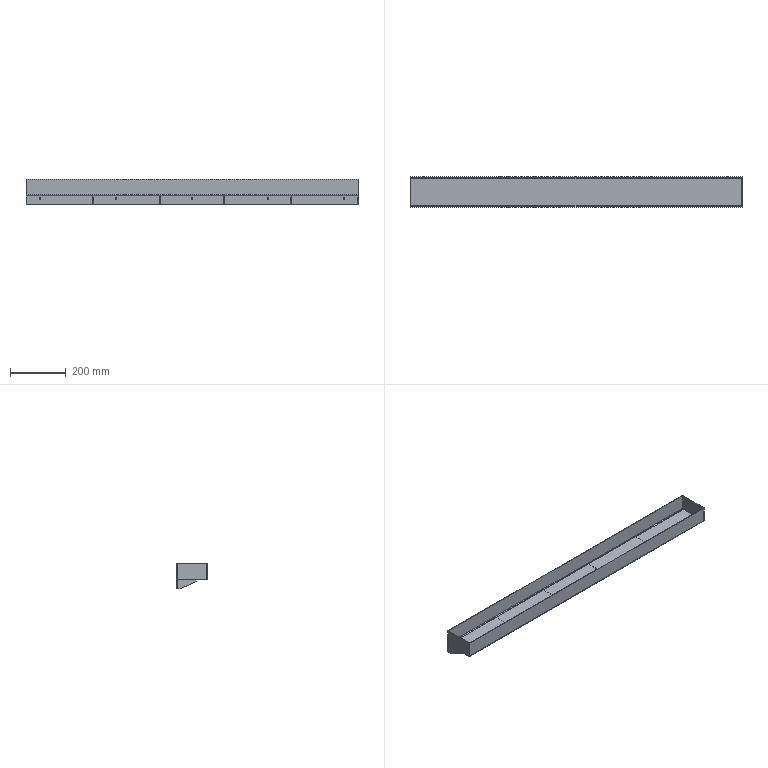Part | STEP file | Sheet metal material box large | 1 solid | 57 faces | box 1190 x 110 x 92 mm | volume 652065 mm3 | plane 39 | cylinder 18 | commonest cylinder face diameters 6.5 x10 10 x6 6 x2